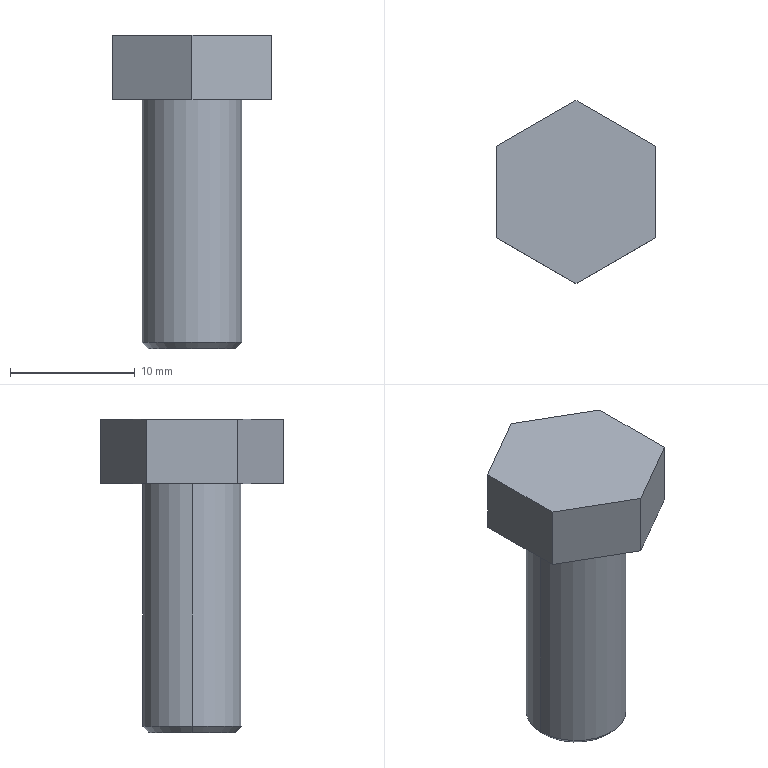Part | STEP file | Bulong M8_2F | 1 solid | 13 faces | box 12.73 x 14.699 x 25.15 mm | volume 1725 mm3 | plane 9 | cone 2 | cylinder 2 | commonest cylinder face diameters 8 x2
STEP:
#1=CARTESIAN_POINT('',(0.,0.,0.));
#2=DIRECTION('',(0.,0.,1.));
#3=DIRECTION('',(1.,0.,0.));
#4=AXIS2_PLACEMENT_3D('',#1,#2,#3);
#5=CARTESIAN_POINT('',(-3.5,0.,-20.));
#6=VERTEX_POINT('',#5);
#7=CARTESIAN_POINT('',(3.5,0.,-20.));
#8=VERTEX_POINT('',#7);
#9=CARTESIAN_POINT('',(0.,0.,-20.));
#10=DIRECTION('',(0.,0.,-1.));
#11=DIRECTION('',(-1.,0.,0.));
#12=AXIS2_PLACEMENT_3D('',#9,#10,#11);
#13=CIRCLE('',#12,3.5);
#14=CARTESIAN_POINT('',(0.,0.,-20.));
#15=DIRECTION('',(0.,0.,1.));
#16=DIRECTION('',(1.,0.,0.));
#17=AXIS2_PLACEMENT_3D('',#14,#15,#16);
#18=CONICAL_SURFACE('',#17,3.5,0.7854);
#19=CARTESIAN_POINT('',(3.142,0.));
#20=DIRECTION('',(-1.,0.));
#21=VECTOR('',#20,1.);
#22=LINE('',#19,#21);
#23=(GEOMETRIC_REPRESENTATION_CONTEXT(2)PARAMETRIC_REPRESENTATION_CONTEXT()REPRESENTATION_CONTEXT('',''));
#24=DEFINITIONAL_REPRESENTATION('',(#22),#23);
#25=PCURVE('',#18,#24);
#26=CARTESIAN_POINT('',(0.,0.,-20.));
#27=DIRECTION('',(0.,0.,-1.));
#28=DIRECTION('',(-1.,0.,0.));
#29=AXIS2_PLACEMENT_3D('',#26,#27,#28);
#30=PLANE('',#29);
#31=CARTESIAN_POINT('',(0.,0.));
#32=DIRECTION('',(1.,0.));
#33=AXIS2_PLACEMENT_2D('',#31,#32);
#34=CIRCLE('',#33,3.5);
#35=(GEOMETRIC_REPRESENTATION_CONTEXT(2)PARAMETRIC_REPRESENTATION_CONTEXT()REPRESENTATION_CONTEXT('',''));
#36=DEFINITIONAL_REPRESENTATION('',(#34),#35);
#37=PCURVE('',#30,#36);
#38=SURFACE_CURVE('',#13,(#25,#37),.PCURVE_S1.);
#39=EDGE_CURVE('',#6,#8,#38,.T.);
#40=ORIENTED_EDGE('',*,*,#39,.F.);
#41=CARTESIAN_POINT('',(-4.,0.,-19.5));
#42=VERTEX_POINT('',#41);
#43=CARTESIAN_POINT('',(-3.5,0.,-20.));
#44=DIRECTION('',(-0.7071,0.,0.7071));
#45=VECTOR('',#44,1.);
#46=LINE('',#43,#45);
#47=CARTESIAN_POINT('',(3.142,0.));
#48=DIRECTION('',(0.,1.));
#49=VECTOR('',#48,1.);
#50=LINE('',#47,#49);
#51=(GEOMETRIC_REPRESENTATION_CONTEXT(2)PARAMETRIC_REPRESENTATION_CONTEXT()REPRESENTATION_CONTEXT('',''));
#52=DEFINITIONAL_REPRESENTATION('',(#50),#51);
#53=PCURVE('',#18,#52);
#54=CARTESIAN_POINT('',(0.,0.,-20.));
#55=DIRECTION('',(0.,0.,1.));
#56=DIRECTION('',(1.,0.,0.));
#57=AXIS2_PLACEMENT_3D('',#54,#55,#56);
#58=CONICAL_SURFACE('',#57,3.5,0.7854);
#59=CARTESIAN_POINT('',(3.142,0.));
#60=DIRECTION('',(0.,1.));
#61=VECTOR('',#60,1.);
#62=LINE('',#59,#61);
#63=(GEOMETRIC_REPRESENTATION_CONTEXT(2)PARAMETRIC_REPRESENTATION_CONTEXT()REPRESENTATION_CONTEXT('',''));
#64=DEFINITIONAL_REPRESENTATION('',(#62),#63);
#65=PCURVE('',#58,#64);
#66=SURFACE_CURVE('',#46,(#53,#65),.PCURVE_S1.);
#67=EDGE_CURVE('',#6,#42,#66,.T.);
#68=ORIENTED_EDGE('',*,*,#67,.T.);
#69=CARTESIAN_POINT('',(4.,0.,-19.5));
#70=VERTEX_POINT('',#69);
#71=CARTESIAN_POINT('',(0.,0.,-19.5));
#72=DIRECTION('',(0.,0.,1.));
#73=DIRECTION('',(-1.,0.,0.));
#74=AXIS2_PLACEMENT_3D('',#71,#72,#73);
#75=CIRCLE('',#74,4.);
#76=CARTESIAN_POINT('',(-3.142,0.5));
#77=DIRECTION('',(1.,0.));
#78=VECTOR('',#77,1.);
#79=LINE('',#76,#78);
#80=(GEOMETRIC_REPRESENTATION_CONTEXT(2)PARAMETRIC_REPRESENTATION_CONTEXT()REPRESENTATION_CONTEXT('',''));
#81=DEFINITIONAL_REPRESENTATION('',(#79),#80);
#82=PCURVE('',#18,#81);
#83=CARTESIAN_POINT('',(0.,0.,-20.));
#84=DIRECTION('',(0.,0.,1.));
#85=DIRECTION('',(1.,0.,0.));
#86=AXIS2_PLACEMENT_3D('',#83,#84,#85);
#87=CYLINDRICAL_SURFACE('',#86,4.);
#88=CARTESIAN_POINT('',(-3.142,0.5));
#89=DIRECTION('',(1.,0.));
#90=VECTOR('',#89,1.);
#91=LINE('',#88,#90);
#92=(GEOMETRIC_REPRESENTATION_CONTEXT(2)PARAMETRIC_REPRESENTATION_CONTEXT()REPRESENTATION_CONTEXT('',''));
#93=DEFINITIONAL_REPRESENTATION('',(#91),#92);
#94=PCURVE('',#87,#93);
#95=SURFACE_CURVE('',#75,(#82,#94),.PCURVE_S1.);
#96=EDGE_CURVE('',#70,#42,#95,.T.);
#97=ORIENTED_EDGE('',*,*,#96,.F.);
#98=CARTESIAN_POINT('',(3.5,0.,-20.));
#99=DIRECTION('',(0.7071,0.,0.7071));
#100=VECTOR('',#99,1.);
#101=LINE('',#98,#100);
#102=CARTESIAN_POINT('',(0.,0.));
#103=DIRECTION('',(0.,1.));
#104=VECTOR('',#103,1.);
#105=LINE('',#102,#104);
#106=(GEOMETRIC_REPRESENTATION_CONTEXT(2)PARAMETRIC_REPRESENTATION_CONTEXT()REPRESENTATION_CONTEXT('',''));
#107=DEFINITIONAL_REPRESENTATION('',(#105),#106);
#108=PCURVE('',#18,#107);
#109=CARTESIAN_POINT('',(6.283,0.));
#110=DIRECTION('',(0.,1.));
#111=VECTOR('',#110,1.);
#112=LINE('',#109,#111);
#113=(GEOMETRIC_REPRESENTATION_CONTEXT(2)PARAMETRIC_REPRESENTATION_CONTEXT()REPRESENTATION_CONTEXT('',''));
#114=DEFINITIONAL_REPRESENTATION('',(#112),#113);
#115=PCURVE('',#58,#114);
#116=SURFACE_CURVE('',#101,(#108,#115),.PCURVE_S1.);
#117=EDGE_CURVE('',#8,#70,#116,.T.);
#118=ORIENTED_EDGE('',*,*,#117,.F.);
#119=EDGE_LOOP('',(#40,#68,#97,#118));
#120=FACE_BOUND('',#119,.T.);
#121=ADVANCED_FACE('',(#120),#18,.T.);
#122=ORIENTED_EDGE('',*,*,#96,.T.);
#123=CARTESIAN_POINT('',(-4.,0.,0.));
#124=VERTEX_POINT('',#123);
#125=CARTESIAN_POINT('',(-4.,0.,-20.));
#126=DIRECTION('',(0.,0.,1.));
#127=VECTOR('',#126,1.);
#128=LINE('',#125,#127);
#129=CARTESIAN_POINT('',(3.142,0.));
#130=DIRECTION('',(0.,1.));
#131=VECTOR('',#130,1.);
#132=LINE('',#129,#131);
#133=(GEOMETRIC_REPRESENTATION_CONTEXT(2)PARAMETRIC_REPRESENTATION_CONTEXT()REPRESENTATION_CONTEXT('',''));
#134=DEFINITIONAL_REPRESENTATION('',(#132),#133);
#135=PCURVE('',#87,#134);
#136=CARTESIAN_POINT('',(0.,0.,-20.));
#137=DIRECTION('',(0.,0.,1.));
#138=DIRECTION('',(1.,0.,0.));
#139=AXIS2_PLACEMENT_3D('',#136,#137,#138);
#140=CYLINDRICAL_SURFACE('',#139,4.);
#141=CARTESIAN_POINT('',(3.142,0.));
#142=DIRECTION('',(0.,1.));
#143=VECTOR('',#142,1.);
#144=LINE('',#141,#143);
#145=(GEOMETRIC_REPRESENTATION_CONTEXT(2)PARAMETRIC_REPRESENTATION_CONTEXT()REPRESENTATION_CONTEXT('',''));
#146=DEFINITIONAL_REPRESENTATION('',(#144),#145);
#147=PCURVE('',#140,#146);
#148=SURFACE_CURVE('',#128,(#135,#147),.PCURVE_S1.);
#149=EDGE_CURVE('',#42,#124,#148,.T.);
#150=ORIENTED_EDGE('',*,*,#149,.T.);
#151=CARTESIAN_POINT('',(4.,0.,0.));
#152=VERTEX_POINT('',#151);
#153=CARTESIAN_POINT('',(0.,0.,0.));
#154=DIRECTION('',(0.,0.,-1.));
#155=DIRECTION('',(1.,0.,0.));
#156=AXIS2_PLACEMENT_3D('',#153,#154,#155);
#157=CIRCLE('',#156,4.);
#158=CARTESIAN_POINT('',(6.283,20.));
#159=DIRECTION('',(-1.,0.));
#160=VECTOR('',#159,1.);
#161=LINE('',#158,#160);
#162=(GEOMETRIC_REPRESENTATION_CONTEXT(2)PARAMETRIC_REPRESENTATION_CONTEXT()REPRESENTATION_CONTEXT('',''));
#163=DEFINITIONAL_REPRESENTATION('',(#161),#162);
#164=PCURVE('',#87,#163);
#165=CARTESIAN_POINT('',(0.,0.,0.));
#166=DIRECTION('',(0.,0.,1.));
#167=DIRECTION('',(1.,0.,0.));
#168=AXIS2_PLACEMENT_3D('',#165,#166,#167);
#169=PLANE('',#168);
#170=CARTESIAN_POINT('',(4.,0.));
#171=CARTESIAN_POINT('',(4.,-6.928));
#172=CARTESIAN_POINT('',(-2.,-3.464));
#173=CARTESIAN_POINT('',(-8.,0.));
#174=CARTESIAN_POINT('',(-2.,3.464));
#175=CARTESIAN_POINT('',(4.,6.928));
#176=CARTESIAN_POINT('',(4.,0.));
#177=(BOUNDED_CURVE()B_SPLINE_CURVE(2,(#170,#171,#172,#173,#174,#175,#176),.UNSPECIFIED.,.T.,.F.)B_SPLINE_CURVE_WITH_KNOTS((1,2,2,2,2,1),(-2.094,0.,2.094,4.189,6.283,8.378),.UNSPECIFIED.)CURVE()GEOMETRIC_REPRESENTATION_ITEM()RATIONAL_B_SPLINE_CURVE((1.,0.5,1.,0.5,1.,0.5,1.))REPRESENTATION_ITEM(''));
#178=(GEOMETRIC_REPRESENTATION_CONTEXT(2)PARAMETRIC_REPRESENTATION_CONTEXT()REPRESENTATION_CONTEXT('',''));
#179=DEFINITIONAL_REPRESENTATION('',(#177),#178);
#180=PCURVE('',#169,#179);
#181=SURFACE_CURVE('',#157,(#164,#180),.PCURVE_S1.);
#182=EDGE_CURVE('',#124,#152,#181,.T.);
#183=ORIENTED_EDGE('',*,*,#182,.T.);
#184=CARTESIAN_POINT('',(4.,0.,-20.));
#185=DIRECTION('',(0.,0.,1.));
#186=VECTOR('',#185,1.);
#187=LINE('',#184,#186);
#188=CARTESIAN_POINT('',(0.,0.));
#189=DIRECTION('',(0.,1.));
#190=VECTOR('',#189,1.);
#191=LINE('',#188,#190);
#192=(GEOMETRIC_REPRESENTATION_CONTEXT(2)PARAMETRIC_REPRESENTATION_CONTEXT()REPRESENTATION_CONTEXT('',''));
#193=DEFINITIONAL_REPRESENTATION('',(#191),#192);
#194=PCURVE('',#87,#193);
#195=CARTESIAN_POINT('',(6.283,0.));
#196=DIRECTION('',(0.,1.));
#197=VECTOR('',#196,1.);
#198=LINE('',#195,#197);
#199=(GEOMETRIC_REPRESENTATION_CONTEXT(2)PARAMETRIC_REPRESENTATION_CONTEXT()REPRESENTATION_CONTEXT('',''));
#200=DEFINITIONAL_REPRESENTATION('',(#198),#199);
#201=PCURVE('',#140,#200);
#202=SURFACE_CURVE('',#187,(#194,#201),.PCURVE_S1.);
#203=EDGE_CURVE('',#70,#152,#202,.T.);
#204=ORIENTED_EDGE('',*,*,#203,.F.);
#205=EDGE_LOOP('',(#122,#150,#183,#204));
#206=FACE_BOUND('',#205,.T.);
#207=ADVANCED_FACE('',(#206),#87,.T.);
#208=CARTESIAN_POINT('',(6.365,3.675,0.));
#209=VERTEX_POINT('',#208);
#210=CARTESIAN_POINT('',(0.,7.35,0.));
#211=VERTEX_POINT('',#210);
#212=CARTESIAN_POINT('',(6.365,3.675,0.));
#213=DIRECTION('',(-0.866,0.5,0.));
#214=VECTOR('',#213,1.);
#215=LINE('',#212,#214);
#216=CARTESIAN_POINT('',(6.365,3.675));
#217=DIRECTION('',(-0.866,0.5));
#218=VECTOR('',#217,1.);
#219=LINE('',#216,#218);
#220=(GEOMETRIC_REPRESENTATION_CONTEXT(2)PARAMETRIC_REPRESENTATION_CONTEXT()REPRESENTATION_CONTEXT('',''));
#221=DEFINITIONAL_REPRESENTATION('',(#219),#220);
#222=PCURVE('',#169,#221);
#223=CARTESIAN_POINT('',(6.365,3.675,5.15));
#224=DIRECTION('',(-0.5,-0.866,0.));
#225=DIRECTION('',(0.866,-0.5,0.));
#226=AXIS2_PLACEMENT_3D('',#223,#224,#225);
#227=PLANE('',#226);
#228=CARTESIAN_POINT('',(0.,-5.15));
#229=DIRECTION('',(-1.,0.));
#230=VECTOR('',#229,1.);
#231=LINE('',#228,#230);
#232=(GEOMETRIC_REPRESENTATION_CONTEXT(2)PARAMETRIC_REPRESENTATION_CONTEXT()REPRESENTATION_CONTEXT('',''));
#233=DEFINITIONAL_REPRESENTATION('',(#231),#232);
#234=PCURVE('',#227,#233);
#235=SURFACE_CURVE('',#215,(#222,#234),.PCURVE_S1.);
#236=EDGE_CURVE('',#209,#211,#235,.T.);
#237=ORIENTED_EDGE('',*,*,#236,.F.);
#238=CARTESIAN_POINT('',(6.365,-3.675,0.));
#239=VERTEX_POINT('',#238);
#240=CARTESIAN_POINT('',(6.365,-3.675,0.));
#241=DIRECTION('',(0.,1.,0.));
#242=VECTOR('',#241,1.);
#243=LINE('',#240,#242);
#244=CARTESIAN_POINT('',(6.365,-3.675));
#245=DIRECTION('',(0.,1.));
#246=VECTOR('',#245,1.);
#247=LINE('',#244,#246);
#248=(GEOMETRIC_REPRESENTATION_CONTEXT(2)PARAMETRIC_REPRESENTATION_CONTEXT()REPRESENTATION_CONTEXT('',''));
#249=DEFINITIONAL_REPRESENTATION('',(#247),#248);
#250=PCURVE('',#169,#249);
#251=CARTESIAN_POINT('',(6.365,-3.675,5.15));
#252=DIRECTION('',(-1.,0.,0.));
#253=DIRECTION('',(0.,-1.,0.));
#254=AXIS2_PLACEMENT_3D('',#251,#252,#253);
#255=PLANE('',#254);
#256=CARTESIAN_POINT('',(0.,-5.15));
#257=DIRECTION('',(-1.,0.));
#258=VECTOR('',#257,1.);
#259=LINE('',#256,#258);
#260=(GEOMETRIC_REPRESENTATION_CONTEXT(2)PARAMETRIC_REPRESENTATION_CONTEXT()REPRESENTATION_CONTEXT('',''));
#261=DEFINITIONAL_REPRESENTATION('',(#259),#260);
#262=PCURVE('',#255,#261);
#263=SURFACE_CURVE('',#243,(#250,#262),.PCURVE_S1.);
#264=EDGE_CURVE('',#239,#209,#263,.T.);
#265=ORIENTED_EDGE('',*,*,#264,.F.);
#266=CARTESIAN_POINT('',(0.,-7.35,0.));
#267=VERTEX_POINT('',#266);
#268=CARTESIAN_POINT('',(0.,-7.35,0.));
#269=DIRECTION('',(0.866,0.5,0.));
#270=VECTOR('',#269,1.);
#271=LINE('',#268,#270);
#272=CARTESIAN_POINT('',(0.,-7.35));
#273=DIRECTION('',(0.866,0.5));
#274=VECTOR('',#273,1.);
#275=LINE('',#272,#274);
#276=(GEOMETRIC_REPRESENTATION_CONTEXT(2)PARAMETRIC_REPRESENTATION_CONTEXT()REPRESENTATION_CONTEXT('',''));
#277=DEFINITIONAL_REPRESENTATION('',(#275),#276);
#278=PCURVE('',#169,#277);
#279=CARTESIAN_POINT('',(0.,-7.35,5.15));
#280=DIRECTION('',(-0.5,0.866,0.));
#281=DIRECTION('',(-0.866,-0.5,0.));
#282=AXIS2_PLACEMENT_3D('',#279,#280,#281);
#283=PLANE('',#282);
#284=CARTESIAN_POINT('',(0.,-5.15));
#285=DIRECTION('',(-1.,0.));
#286=VECTOR('',#285,1.);
#287=LINE('',#284,#286);
#288=(GEOMETRIC_REPRESENTATION_CONTEXT(2)PARAMETRIC_REPRESENTATION_CONTEXT()REPRESENTATION_CONTEXT('',''));
#289=DEFINITIONAL_REPRESENTATION('',(#287),#288);
#290=PCURVE('',#283,#289);
#291=SURFACE_CURVE('',#271,(#278,#290),.PCURVE_S1.);
#292=EDGE_CURVE('',#267,#239,#291,.T.);
#293=ORIENTED_EDGE('',*,*,#292,.F.);
#294=CARTESIAN_POINT('',(-6.365,-3.675,0.));
#295=VERTEX_POINT('',#294);
#296=CARTESIAN_POINT('',(-6.365,-3.675,0.));
#297=DIRECTION('',(0.866,-0.5,0.));
#298=VECTOR('',#297,1.);
#299=LINE('',#296,#298);
#300=CARTESIAN_POINT('',(-6.365,-3.675));
#301=DIRECTION('',(0.866,-0.5));
#302=VECTOR('',#301,1.);
#303=LINE('',#300,#302);
#304=(GEOMETRIC_REPRESENTATION_CONTEXT(2)PARAMETRIC_REPRESENTATION_CONTEXT()REPRESENTATION_CONTEXT('',''));
#305=DEFINITIONAL_REPRESENTATION('',(#303),#304);
#306=PCURVE('',#169,#305);
#307=CARTESIAN_POINT('',(-6.365,-3.675,5.15));
#308=DIRECTION('',(0.5,0.866,0.));
#309=DIRECTION('',(-0.866,0.5,0.));
#310=AXIS2_PLACEMENT_3D('',#307,#308,#309);
#311=PLANE('',#310);
#312=CARTESIAN_POINT('',(0.,-5.15));
#313=DIRECTION('',(-1.,0.));
#314=VECTOR('',#313,1.);
#315=LINE('',#312,#314);
#316=(GEOMETRIC_REPRESENTATION_CONTEXT(2)PARAMETRIC_REPRESENTATION_CONTEXT()REPRESENTATION_CONTEXT('',''));
#317=DEFINITIONAL_REPRESENTATION('',(#315),#316);
#318=PCURVE('',#311,#317);
#319=SURFACE_CURVE('',#299,(#306,#318),.PCURVE_S1.);
#320=EDGE_CURVE('',#295,#267,#319,.T.);
#321=ORIENTED_EDGE('',*,*,#320,.F.);
#322=CARTESIAN_POINT('',(-6.365,3.675,0.));
#323=VERTEX_POINT('',#322);
#324=CARTESIAN_POINT('',(-6.365,3.675,0.));
#325=DIRECTION('',(0.,-1.,0.));
#326=VECTOR('',#325,1.);
#327=LINE('',#324,#326);
#328=CARTESIAN_POINT('',(-6.365,3.675));
#329=DIRECTION('',(0.,-1.));
#330=VECTOR('',#329,1.);
#331=LINE('',#328,#330);
#332=(GEOMETRIC_REPRESENTATION_CONTEXT(2)PARAMETRIC_REPRESENTATION_CONTEXT()REPRESENTATION_CONTEXT('',''));
#333=DEFINITIONAL_REPRESENTATION('',(#331),#332);
#334=PCURVE('',#169,#333);
#335=CARTESIAN_POINT('',(-6.365,3.675,5.15));
#336=DIRECTION('',(1.,0.,0.));
#337=DIRECTION('',(0.,0.,-1.));
#338=AXIS2_PLACEMENT_3D('',#335,#336,#337);
#339=PLANE('',#338);
#340=CARTESIAN_POINT('',(5.15,0.));
#341=DIRECTION('',(0.,-1.));
#342=VECTOR('',#341,1.);
#343=LINE('',#340,#342);
#344=(GEOMETRIC_REPRESENTATION_CONTEXT(2)PARAMETRIC_REPRESENTATION_CONTEXT()REPRESENTATION_CONTEXT('',''));
#345=DEFINITIONAL_REPRESENTATION('',(#343),#344);
#346=PCURVE('',#339,#345);
#347=SURFACE_CURVE('',#327,(#334,#346),.PCURVE_S1.);
#348=EDGE_CURVE('',#323,#295,#347,.T.);
#349=ORIENTED_EDGE('',*,*,#348,.F.);
#350=CARTESIAN_POINT('',(0.,7.35,0.));
#351=DIRECTION('',(-0.866,-0.5,0.));
#352=VECTOR('',#351,1.);
#353=LINE('',#350,#352);
#354=CARTESIAN_POINT('',(0.,7.35));
#355=DIRECTION('',(-0.866,-0.5));
#356=VECTOR('',#355,1.);
#357=LINE('',#354,#356);
#358=(GEOMETRIC_REPRESENTATION_CONTEXT(2)PARAMETRIC_REPRESENTATION_CONTEXT()REPRESENTATION_CONTEXT('',''));
#359=DEFINITIONAL_REPRESENTATION('',(#357),#358);
#360=PCURVE('',#169,#359);
#361=CARTESIAN_POINT('',(0.,7.35,5.15));
#362=DIRECTION('',(0.5,-0.866,0.));
#363=DIRECTION('',(0.866,0.5,0.));
#364=AXIS2_PLACEMENT_3D('',#361,#362,#363);
#365=PLANE('',#364);
#366=CARTESIAN_POINT('',(0.,-5.15));
#367=DIRECTION('',(-1.,0.));
#368=VECTOR('',#367,1.);
#369=LINE('',#366,#368);
#370=(GEOMETRIC_REPRESENTATION_CONTEXT(2)PARAMETRIC_REPRESENTATION_CONTEXT()REPRESENTATION_CONTEXT('',''));
#371=DEFINITIONAL_REPRESENTATION('',(#369),#370);
#372=PCURVE('',#365,#371);
#373=SURFACE_CURVE('',#353,(#360,#372),.PCURVE_S1.);
#374=EDGE_CURVE('',#211,#323,#373,.T.);
#375=ORIENTED_EDGE('',*,*,#374,.F.);
#376=EDGE_LOOP('',(#237,#265,#293,#321,#349,#375));
#377=FACE_BOUND('',#376,.T.);
#378=CARTESIAN_POINT('',(0.,0.,0.));
#379=DIRECTION('',(0.,0.,-1.));
#380=DIRECTION('',(1.,0.,0.));
#381=AXIS2_PLACEMENT_3D('',#378,#379,#380);
#382=CIRCLE('',#381,4.);
#383=CARTESIAN_POINT('',(4.,0.));
#384=CARTESIAN_POINT('',(4.,-6.928));
#385=CARTESIAN_POINT('',(-2.,-3.464));
#386=CARTESIAN_POINT('',(-8.,0.));
#387=CARTESIAN_POINT('',(-2.,3.464));
#388=CARTESIAN_POINT('',(4.,6.928));
#389=CARTESIAN_POINT('',(4.,0.));
#390=(BOUNDED_CURVE()B_SPLINE_CURVE(2,(#383,#384,#385,#386,#387,#388,#389),.UNSPECIFIED.,.T.,.F.)B_SPLINE_CURVE_WITH_KNOTS((1,2,2,2,2,1),(-2.094,0.,2.094,4.189,6.283,8.378),.UNSPECIFIED.)CURVE()GEOMETRIC_REPRESENTATION_ITEM()RATIONAL_B_SPLINE_CURVE((1.,0.5,1.,0.5,1.,0.5,1.))REPRESENTATION_ITEM(''));
#391=(GEOMETRIC_REPRESENTATION_CONTEXT(2)PARAMETRIC_REPRESENTATION_CONTEXT()REPRESENTATION_CONTEXT('',''));
#392=DEFINITIONAL_REPRESENTATION('',(#390),#391);
#393=PCURVE('',#169,#392);
#394=CARTESIAN_POINT('',(6.283,20.));
#395=DIRECTION('',(-1.,0.));
#396=VECTOR('',#395,1.);
#397=LINE('',#394,#396);
#398=(GEOMETRIC_REPRESENTATION_CONTEXT(2)PARAMETRIC_REPRESENTATION_CONTEXT()REPRESENTATION_CONTEXT('',''));
#399=DEFINITIONAL_REPRESENTATION('',(#397),#398);
#400=PCURVE('',#140,#399);
#401=SURFACE_CURVE('',#382,(#393,#400),.PCURVE_S1.);
#402=EDGE_CURVE('',#152,#124,#401,.T.);
#403=ORIENTED_EDGE('',*,*,#402,.F.);
#404=ORIENTED_EDGE('',*,*,#182,.F.);
#405=EDGE_LOOP('',(#403,#404));
#406=FACE_BOUND('',#405,.T.);
#407=ADVANCED_FACE('',(#377,#406),#169,.F.);
#408=ORIENTED_EDGE('',*,*,#236,.T.);
#409=CARTESIAN_POINT('',(0.,7.35,5.15));
#410=VERTEX_POINT('',#409);
#411=CARTESIAN_POINT('',(0.,7.35,5.15));
#412=DIRECTION('',(0.,0.,-1.));
#413=VECTOR('',#412,1.);
#414=LINE('',#411,#413);
#415=CARTESIAN_POINT('',(-7.35,0.));
#416=DIRECTION('',(0.,-1.));
#417=VECTOR('',#416,1.);
#418=LINE('',#415,#417);
#419=(GEOMETRIC_REPRESENTATION_CONTEXT(2)PARAMETRIC_REPRESENTATION_CONTEXT()REPRESENTATION_CONTEXT('',''));
#420=DEFINITIONAL_REPRESENTATION('',(#418),#419);
#421=PCURVE('',#227,#420);
#422=CARTESIAN_POINT('',(0.,0.));
#423=DIRECTION('',(0.,-1.));
#424=VECTOR('',#423,1.);
#425=LINE('',#422,#424);
#426=(GEOMETRIC_REPRESENTATION_CONTEXT(2)PARAMETRIC_REPRESENTATION_CONTEXT()REPRESENTATION_CONTEXT('',''));
#427=DEFINITIONAL_REPRESENTATION('',(#425),#426);
#428=PCURVE('',#365,#427);
#429=SURFACE_CURVE('',#414,(#421,#428),.PCURVE_S1.);
#430=EDGE_CURVE('',#410,#211,#429,.T.);
#431=ORIENTED_EDGE('',*,*,#430,.F.);
#432=CARTESIAN_POINT('',(6.365,3.675,5.15));
#433=VERTEX_POINT('',#432);
#434=CARTESIAN_POINT('',(6.365,3.675,5.15));
#435=DIRECTION('',(-0.866,0.5,0.));
#436=VECTOR('',#435,1.);
#437=LINE('',#434,#436);
#438=CARTESIAN_POINT('',(0.,0.));
#439=DIRECTION('',(-1.,0.));
#440=VECTOR('',#439,1.);
#441=LINE('',#438,#440);
#442=(GEOMETRIC_REPRESENTATION_CONTEXT(2)PARAMETRIC_REPRESENTATION_CONTEXT()REPRESENTATION_CONTEXT('',''));
#443=DEFINITIONAL_REPRESENTATION('',(#441),#442);
#444=PCURVE('',#227,#443);
#445=CARTESIAN_POINT('',(0.,0.,5.15));
#446=DIRECTION('',(0.,0.,1.));
#447=DIRECTION('',(1.,0.,0.));
#448=AXIS2_PLACEMENT_3D('',#445,#446,#447);
#449=PLANE('',#448);
#450=CARTESIAN_POINT('',(6.365,3.675));
#451=DIRECTION('',(-0.866,0.5));
#452=VECTOR('',#451,1.);
#453=LINE('',#450,#452);
#454=(GEOMETRIC_REPRESENTATION_CONTEXT(2)PARAMETRIC_REPRESENTATION_CONTEXT()REPRESENTATION_CONTEXT('',''));
#455=DEFINITIONAL_REPRESENTATION('',(#453),#454);
#456=PCURVE('',#449,#455);
#457=SURFACE_CURVE('',#437,(#444,#456),.PCURVE_S1.);
#458=EDGE_CURVE('',#433,#410,#457,.T.);
#459=ORIENTED_EDGE('',*,*,#458,.F.);
#460=CARTESIAN_POINT('',(6.365,3.675,5.15));
#461=DIRECTION('',(0.,0.,-1.));
#462=VECTOR('',#461,1.);
#463=LINE('',#460,#462);
#464=CARTESIAN_POINT('',(0.,0.));
#465=DIRECTION('',(0.,-1.));
#466=VECTOR('',#465,1.);
#467=LINE('',#464,#466);
#468=(GEOMETRIC_REPRESENTATION_CONTEXT(2)PARAMETRIC_REPRESENTATION_CONTEXT()REPRESENTATION_CONTEXT('',''));
#469=DEFINITIONAL_REPRESENTATION('',(#467),#468);
#470=PCURVE('',#227,#469);
#471=CARTESIAN_POINT('',(-7.35,0.));
#472=DIRECTION('',(0.,-1.));
#473=VECTOR('',#472,1.);
#474=LINE('',#471,#473);
#475=(GEOMETRIC_REPRESENTATION_CONTEXT(2)PARAMETRIC_REPRESENTATION_CONTEXT()REPRESENTATION_CONTEXT('',''));
#476=DEFINITIONAL_REPRESENTATION('',(#474),#475);
#477=PCURVE('',#255,#476);
#478=SURFACE_CURVE('',#463,(#470,#477),.PCURVE_S1.);
#479=EDGE_CURVE('',#433,#209,#478,.T.);
#480=ORIENTED_EDGE('',*,*,#479,.T.);
#481=EDGE_LOOP('',(#408,#431,#459,#480));
#482=FACE_BOUND('',#481,.T.);
#483=ADVANCED_FACE('',(#482),#227,.F.);
#484=ORIENTED_EDGE('',*,*,#374,.T.);
#485=CARTESIAN_POINT('',(-6.365,3.675,5.15));
#486=VERTEX_POINT('',#485);
#487=CARTESIAN_POINT('',(-6.365,3.675,5.15));
#488=DIRECTION('',(0.,0.,-1.));
#489=VECTOR('',#488,1.);
#490=LINE('',#487,#489);
#491=CARTESIAN_POINT('',(-7.35,0.));
#492=DIRECTION('',(0.,-1.));
#493=VECTOR('',#492,1.);
#494=LINE('',#491,#493);
#495=(GEOMETRIC_REPRESENTATION_CONTEXT(2)PARAMETRIC_REPRESENTATION_CONTEXT()REPRESENTATION_CONTEXT('',''));
#496=DEFINITIONAL_REPRESENTATION('',(#494),#495);
#497=PCURVE('',#365,#496);
#498=CARTESIAN_POINT('',(0.,0.));
#499=DIRECTION('',(1.,0.));
#500=VECTOR('',#499,1.);
#501=LINE('',#498,#500);
#502=(GEOMETRIC_REPRESENTATION_CONTEXT(2)PARAMETRIC_REPRESENTATION_CONTEXT()REPRESENTATION_CONTEXT('',''));
#503=DEFINITIONAL_REPRESENTATION('',(#501),#502);
#504=PCURVE('',#339,#503);
#505=SURFACE_CURVE('',#490,(#497,#504),.PCURVE_S1.);
#506=EDGE_CURVE('',#486,#323,#505,.T.);
#507=ORIENTED_EDGE('',*,*,#506,.F.);
#508=CARTESIAN_POINT('',(0.,7.35,5.15));
#509=DIRECTION('',(-0.866,-0.5,0.));
#510=VECTOR('',#509,1.);
#511=LINE('',#508,#510);
#512=CARTESIAN_POINT('',(0.,0.));
#513=DIRECTION('',(-1.,0.));
#514=VECTOR('',#513,1.);
#515=LINE('',#512,#514);
#516=(GEOMETRIC_REPRESENTATION_CONTEXT(2)PARAMETRIC_REPRESENTATION_CONTEXT()REPRESENTATION_CONTEXT('',''));
#517=DEFINITIONAL_REPRESENTATION('',(#515),#516);
#518=PCURVE('',#365,#517);
#519=CARTESIAN_POINT('',(0.,7.35));
#520=DIRECTION('',(-0.866,-0.5));
#521=VECTOR('',#520,1.);
#522=LINE('',#519,#521);
#523=(GEOMETRIC_REPRESENTATION_CONTEXT(2)PARAMETRIC_REPRESENTATION_CONTEXT()REPRESENTATION_CONTEXT('',''));
#524=DEFINITIONAL_REPRESENTATION('',(#522),#523);
#525=PCURVE('',#449,#524);
#526=SURFACE_CURVE('',#511,(#518,#525),.PCURVE_S1.);
#527=EDGE_CURVE('',#410,#486,#526,.T.);
#528=ORIENTED_EDGE('',*,*,#527,.F.);
#529=ORIENTED_EDGE('',*,*,#430,.T.);
#530=EDGE_LOOP('',(#484,#507,#528,#529));
#531=FACE_BOUND('',#530,.T.);
#532=ADVANCED_FACE('',(#531),#365,.F.);
#533=ORIENTED_EDGE('',*,*,#348,.T.);
#534=CARTESIAN_POINT('',(-6.365,-3.675,5.15));
#535=VERTEX_POINT('',#534);
#536=CARTESIAN_POINT('',(-6.365,-3.675,5.15));
#537=DIRECTION('',(0.,0.,-1.));
#538=VECTOR('',#537,1.);
#539=LINE('',#536,#538);
#540=CARTESIAN_POINT('',(0.,-7.35));
#541=DIRECTION('',(1.,0.));
#542=VECTOR('',#541,1.);
#543=LINE('',#540,#542);
#544=(GEOMETRIC_REPRESENTATION_CONTEXT(2)PARAMETRIC_REPRESENTATION_CONTEXT()REPRESENTATION_CONTEXT('',''));
#545=DEFINITIONAL_REPRESENTATION('',(#543),#544);
#546=PCURVE('',#339,#545);
#547=CARTESIAN_POINT('',(0.,0.));
#548=DIRECTION('',(0.,-1.));
#549=VECTOR('',#548,1.);
#550=LINE('',#547,#549);
#551=(GEOMETRIC_REPRESENTATION_CONTEXT(2)PARAMETRIC_REPRESENTATION_CONTEXT()REPRESENTATION_CONTEXT('',''));
#552=DEFINITIONAL_REPRESENTATION('',(#550),#551);
#553=PCURVE('',#311,#552);
#554=SURFACE_CURVE('',#539,(#546,#553),.PCURVE_S1.);
#555=EDGE_CURVE('',#535,#295,#554,.T.);
#556=ORIENTED_EDGE('',*,*,#555,.F.);
#557=CARTESIAN_POINT('',(-6.365,3.675,5.15));
#558=DIRECTION('',(0.,-1.,0.));
#559=VECTOR('',#558,1.);
#560=LINE('',#557,#559);
#561=CARTESIAN_POINT('',(0.,0.));
#562=DIRECTION('',(0.,-1.));
#563=VECTOR('',#562,1.);
#564=LINE('',#561,#563);
#565=(GEOMETRIC_REPRESENTATION_CONTEXT(2)PARAMETRIC_REPRESENTATION_CONTEXT()REPRESENTATION_CONTEXT('',''));
#566=DEFINITIONAL_REPRESENTATION('',(#564),#565);
#567=PCURVE('',#339,#566);
#568=CARTESIAN_POINT('',(-6.365,3.675));
#569=DIRECTION('',(0.,-1.));
#570=VECTOR('',#569,1.);
#571=LINE('',#568,#570);
#572=(GEOMETRIC_REPRESENTATION_CONTEXT(2)PARAMETRIC_REPRESENTATION_CONTEXT()REPRESENTATION_CONTEXT('',''));
#573=DEFINITIONAL_REPRESENTATION('',(#571),#572);
#574=PCURVE('',#449,#573);
#575=SURFACE_CURVE('',#560,(#567,#574),.PCURVE_S1.);
#576=EDGE_CURVE('',#486,#535,#575,.T.);
#577=ORIENTED_EDGE('',*,*,#576,.F.);
#578=ORIENTED_EDGE('',*,*,#506,.T.);
#579=EDGE_LOOP('',(#533,#556,#577,#578));
#580=FACE_BOUND('',#579,.T.);
#581=ADVANCED_FACE('',(#580),#339,.F.);
#582=ORIENTED_EDGE('',*,*,#320,.T.);
#583=CARTESIAN_POINT('',(0.,-7.35,5.15));
#584=VERTEX_POINT('',#583);
#585=CARTESIAN_POINT('',(0.,-7.35,5.15));
#586=DIRECTION('',(0.,0.,-1.));
#587=VECTOR('',#586,1.);
#588=LINE('',#585,#587);
#589=CARTESIAN_POINT('',(-7.35,0.));
#590=DIRECTION('',(0.,-1.));
#591=VECTOR('',#590,1.);
#592=LINE('',#589,#591);
#593=(GEOMETRIC_REPRESENTATION_CONTEXT(2)PARAMETRIC_REPRESENTATION_CONTEXT()REPRESENTATION_CONTEXT('',''));
#594=DEFINITIONAL_REPRESENTATION('',(#592),#593);
#595=PCURVE('',#311,#594);
#596=CARTESIAN_POINT('',(0.,0.));
#597=DIRECTION('',(0.,-1.));
#598=VECTOR('',#597,1.);
#599=LINE('',#596,#598);
#600=(GEOMETRIC_REPRESENTATION_CONTEXT(2)PARAMETRIC_REPRESENTATION_CONTEXT()REPRESENTATION_CONTEXT('',''));
#601=DEFINITIONAL_REPRESENTATION('',(#599),#600);
#602=PCURVE('',#283,#601);
#603=SURFACE_CURVE('',#588,(#595,#602),.PCURVE_S1.);
#604=EDGE_CURVE('',#584,#267,#603,.T.);
#605=ORIENTED_EDGE('',*,*,#604,.F.);
#606=CARTESIAN_POINT('',(-6.365,-3.675,5.15));
#607=DIRECTION('',(0.866,-0.5,0.));
#608=VECTOR('',#607,1.);
#609=LINE('',#606,#608);
#610=CARTESIAN_POINT('',(0.,0.));
#611=DIRECTION('',(-1.,0.));
#612=VECTOR('',#611,1.);
#613=LINE('',#610,#612);
#614=(GEOMETRIC_REPRESENTATION_CONTEXT(2)PARAMETRIC_REPRESENTATION_CONTEXT()REPRESENTATION_CONTEXT('',''));
#615=DEFINITIONAL_REPRESENTATION('',(#613),#614);
#616=PCURVE('',#311,#615);
#617=CARTESIAN_POINT('',(-6.365,-3.675));
#618=DIRECTION('',(0.866,-0.5));
#619=VECTOR('',#618,1.);
#620=LINE('',#617,#619);
#621=(GEOMETRIC_REPRESENTATION_CONTEXT(2)PARAMETRIC_REPRESENTATION_CONTEXT()REPRESENTATION_CONTEXT('',''));
#622=DEFINITIONAL_REPRESENTATION('',(#620),#621);
#623=PCURVE('',#449,#622);
#624=SURFACE_CURVE('',#609,(#616,#623),.PCURVE_S1.);
#625=EDGE_CURVE('',#535,#584,#624,.T.);
#626=ORIENTED_EDGE('',*,*,#625,.F.);
#627=ORIENTED_EDGE('',*,*,#555,.T.);
#628=EDGE_LOOP('',(#582,#605,#626,#627));
#629=FACE_BOUND('',#628,.T.);
#630=ADVANCED_FACE('',(#629),#311,.F.);
#631=ORIENTED_EDGE('',*,*,#292,.T.);
#632=CARTESIAN_POINT('',(6.365,-3.675,5.15));
#633=VERTEX_POINT('',#632);
#634=CARTESIAN_POINT('',(6.365,-3.675,5.15));
#635=DIRECTION('',(0.,0.,-1.));
#636=VECTOR('',#635,1.);
#637=LINE('',#634,#636);
#638=CARTESIAN_POINT('',(-7.35,0.));
#639=DIRECTION('',(0.,-1.));
#640=VECTOR('',#639,1.);
#641=LINE('',#638,#640);
#642=(GEOMETRIC_REPRESENTATION_CONTEXT(2)PARAMETRIC_REPRESENTATION_CONTEXT()REPRESENTATION_CONTEXT('',''));
#643=DEFINITIONAL_REPRESENTATION('',(#641),#642);
#644=PCURVE('',#283,#643);
#645=CARTESIAN_POINT('',(0.,0.));
#646=DIRECTION('',(0.,-1.));
#647=VECTOR('',#646,1.);
#648=LINE('',#645,#647);
#649=(GEOMETRIC_REPRESENTATION_CONTEXT(2)PARAMETRIC_REPRESENTATION_CONTEXT()REPRESENTATION_CONTEXT('',''));
#650=DEFINITIONAL_REPRESENTATION('',(#648),#649);
#651=PCURVE('',#255,#650);
#652=SURFACE_CURVE('',#637,(#644,#651),.PCURVE_S1.);
#653=EDGE_CURVE('',#633,#239,#652,.T.);
#654=ORIENTED_EDGE('',*,*,#653,.F.);
#655=CARTESIAN_POINT('',(0.,-7.35,5.15));
#656=DIRECTION('',(0.866,0.5,0.));
#657=VECTOR('',#656,1.);
#658=LINE('',#655,#657);
#659=CARTESIAN_POINT('',(0.,0.));
#660=DIRECTION('',(-1.,0.));
#661=VECTOR('',#660,1.);
#662=LINE('',#659,#661);
#663=(GEOMETRIC_REPRESENTATION_CONTEXT(2)PARAMETRIC_REPRESENTATION_CONTEXT()REPRESENTATION_CONTEXT('',''));
#664=DEFINITIONAL_REPRESENTATION('',(#662),#663);
#665=PCURVE('',#283,#664);
#666=CARTESIAN_POINT('',(0.,-7.35));
#667=DIRECTION('',(0.866,0.5));
#668=VECTOR('',#667,1.);
#669=LINE('',#666,#668);
#670=(GEOMETRIC_REPRESENTATION_CONTEXT(2)PARAMETRIC_REPRESENTATION_CONTEXT()REPRESENTATION_CONTEXT('',''));
#671=DEFINITIONAL_REPRESENTATION('',(#669),#670);
#672=PCURVE('',#449,#671);
#673=SURFACE_CURVE('',#658,(#665,#672),.PCURVE_S1.);
#674=EDGE_CURVE('',#584,#633,#673,.T.);
#675=ORIENTED_EDGE('',*,*,#674,.F.);
#676=ORIENTED_EDGE('',*,*,#604,.T.);
#677=EDGE_LOOP('',(#631,#654,#675,#676));
#678=FACE_BOUND('',#677,.T.);
#679=ADVANCED_FACE('',(#678),#283,.F.);
#680=ORIENTED_EDGE('',*,*,#264,.T.);
#681=ORIENTED_EDGE('',*,*,#479,.F.);
#682=CARTESIAN_POINT('',(6.365,-3.675,5.15));
#683=DIRECTION('',(0.,1.,0.));
#684=VECTOR('',#683,1.);
#685=LINE('',#682,#684);
#686=CARTESIAN_POINT('',(0.,0.));
#687=DIRECTION('',(-1.,0.));
#688=VECTOR('',#687,1.);
#689=LINE('',#686,#688);
#690=(GEOMETRIC_REPRESENTATION_CONTEXT(2)PARAMETRIC_REPRESENTATION_CONTEXT()REPRESENTATION_CONTEXT('',''));
#691=DEFINITIONAL_REPRESENTATION('',(#689),#690);
#692=PCURVE('',#255,#691);
#693=CARTESIAN_POINT('',(6.365,-3.675));
#694=DIRECTION('',(0.,1.));
#695=VECTOR('',#694,1.);
#696=LINE('',#693,#695);
#697=(GEOMETRIC_REPRESENTATION_CONTEXT(2)PARAMETRIC_REPRESENTATION_CONTEXT()REPRESENTATION_CONTEXT('',''));
#698=DEFINITIONAL_REPRESENTATION('',(#696),#697);
#699=PCURVE('',#449,#698);
#700=SURFACE_CURVE('',#685,(#692,#699),.PCURVE_S1.);
#701=EDGE_CURVE('',#633,#433,#700,.T.);
#702=ORIENTED_EDGE('',*,*,#701,.F.);
#703=ORIENTED_EDGE('',*,*,#653,.T.);
#704=EDGE_LOOP('',(#680,#681,#702,#703));
#705=FACE_BOUND('',#704,.T.);
#706=ADVANCED_FACE('',(#705),#255,.F.);
#707=ORIENTED_EDGE('',*,*,#458,.T.);
#708=ORIENTED_EDGE('',*,*,#527,.T.);
#709=ORIENTED_EDGE('',*,*,#576,.T.);
#710=ORIENTED_EDGE('',*,*,#625,.T.);
#711=ORIENTED_EDGE('',*,*,#674,.T.);
#712=ORIENTED_EDGE('',*,*,#701,.T.);
#713=EDGE_LOOP('',(#707,#708,#709,#710,#711,#712));
#714=FACE_BOUND('',#713,.T.);
#715=ADVANCED_FACE('',(#714),#449,.T.);
#716=ORIENTED_EDGE('',*,*,#149,.F.);
#717=CARTESIAN_POINT('',(0.,0.,-19.5));
#718=DIRECTION('',(0.,0.,1.));
#719=DIRECTION('',(-1.,0.,0.));
#720=AXIS2_PLACEMENT_3D('',#717,#718,#719);
#721=CIRCLE('',#720,4.);
#722=CARTESIAN_POINT('',(3.142,0.5));
#723=DIRECTION('',(1.,0.));
#724=VECTOR('',#723,1.);
#725=LINE('',#722,#724);
#726=(GEOMETRIC_REPRESENTATION_CONTEXT(2)PARAMETRIC_REPRESENTATION_CONTEXT()REPRESENTATION_CONTEXT('',''));
#727=DEFINITIONAL_REPRESENTATION('',(#725),#726);
#728=PCURVE('',#140,#727);
#729=CARTESIAN_POINT('',(3.142,0.5));
#730=DIRECTION('',(1.,0.));
#731=VECTOR('',#730,1.);
#732=LINE('',#729,#731);
#733=(GEOMETRIC_REPRESENTATION_CONTEXT(2)PARAMETRIC_REPRESENTATION_CONTEXT()REPRESENTATION_CONTEXT('',''));
#734=DEFINITIONAL_REPRESENTATION('',(#732),#733);
#735=PCURVE('',#58,#734);
#736=SURFACE_CURVE('',#721,(#728,#735),.PCURVE_S1.);
#737=EDGE_CURVE('',#42,#70,#736,.T.);
#738=ORIENTED_EDGE('',*,*,#737,.T.);
#739=ORIENTED_EDGE('',*,*,#203,.T.);
#740=ORIENTED_EDGE('',*,*,#402,.T.);
#741=EDGE_LOOP('',(#716,#738,#739,#740));
#742=FACE_BOUND('',#741,.T.);
#743=ADVANCED_FACE('',(#742),#140,.T.);
#744=CARTESIAN_POINT('',(0.,0.,-20.));
#745=DIRECTION('',(0.,0.,-1.));
#746=DIRECTION('',(-1.,0.,0.));
#747=AXIS2_PLACEMENT_3D('',#744,#745,#746);
#748=CIRCLE('',#747,3.5);
#749=CARTESIAN_POINT('',(0.,0.));
#750=DIRECTION('',(1.,0.));
#751=AXIS2_PLACEMENT_2D('',#749,#750);
#752=CIRCLE('',#751,3.5);
#753=(GEOMETRIC_REPRESENTATION_CONTEXT(2)PARAMETRIC_REPRESENTATION_CONTEXT()REPRESENTATION_CONTEXT('',''));
#754=DEFINITIONAL_REPRESENTATION('',(#752),#753);
#755=PCURVE('',#30,#754);
#756=CARTESIAN_POINT('',(9.425,0.));
#757=DIRECTION('',(-1.,0.));
#758=VECTOR('',#757,1.);
#759=LINE('',#756,#758);
#760=(GEOMETRIC_REPRESENTATION_CONTEXT(2)PARAMETRIC_REPRESENTATION_CONTEXT()REPRESENTATION_CONTEXT('',''));
#761=DEFINITIONAL_REPRESENTATION('',(#759),#760);
#762=PCURVE('',#58,#761);
#763=SURFACE_CURVE('',#748,(#755,#762),.PCURVE_S1.);
#764=EDGE_CURVE('',#8,#6,#763,.T.);
#765=ORIENTED_EDGE('',*,*,#764,.T.);
#766=ORIENTED_EDGE('',*,*,#39,.T.);
#767=EDGE_LOOP('',(#765,#766));
#768=FACE_BOUND('',#767,.T.);
#769=ADVANCED_FACE('',(#768),#30,.T.);
#770=ORIENTED_EDGE('',*,*,#67,.F.);
#771=ORIENTED_EDGE('',*,*,#764,.F.);
#772=ORIENTED_EDGE('',*,*,#117,.T.);
#773=ORIENTED_EDGE('',*,*,#737,.F.);
#774=EDGE_LOOP('',(#770,#771,#772,#773));
#775=FACE_BOUND('',#774,.T.);
#776=ADVANCED_FACE('',(#775),#58,.T.);
#777=CLOSED_SHELL('',(#121,#207,#407,#483,#532,#581,#630,#679,#706,#715,#743,#769,#776));
#778=MANIFOLD_SOLID_BREP('',#777);
#779=(LENGTH_UNIT()NAMED_UNIT(*)SI_UNIT(.MILLI.,.METRE.));
#780=UNCERTAINTY_MEASURE_WITH_UNIT(LENGTH_MEASURE(0.0000001),#779,'','');
#781=(NAMED_UNIT(*)PLANE_ANGLE_UNIT()SI_UNIT($,.RADIAN.));
#782=(NAMED_UNIT(*)SI_UNIT($,.STERADIAN.)SOLID_ANGLE_UNIT());
#783=(GEOMETRIC_REPRESENTATION_CONTEXT(3)GLOBAL_UNCERTAINTY_ASSIGNED_CONTEXT((#780))GLOBAL_UNIT_ASSIGNED_CONTEXT((#779,#781,#782))REPRESENTATION_CONTEXT('',''));
#784=ADVANCED_BREP_SHAPE_REPRESENTATION('',(#4,#778),#783);